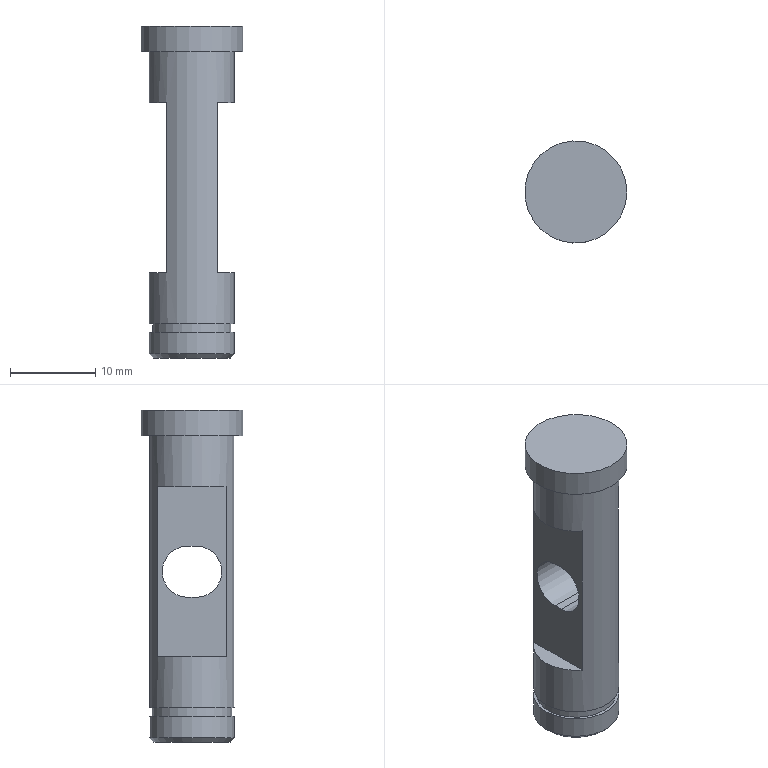Part | NX | features BREP 1, DATUM_CSYS 1 | 1 solid | 20 faces | box 12 x 12 x 39 mm | volume 2499 mm3 | plane 13 | cylinder 6 | cone 1 | commonest cylinder face diameters 6 x2 10 x2 9.3 x1 12 x1
STEP:
#1=CARTESIAN_POINT('',(6.,0.,3.));
#2=VERTEX_POINT('',#1);
#3=CARTESIAN_POINT('',(0.,0.,3.));
#4=DIRECTION('',(0.,0.,1.));
#5=DIRECTION('',(1.,0.,0.));
#6=AXIS2_PLACEMENT_3D('',#3,#4,#5);
#7=CIRCLE('',#6,6.);
#8=EDGE_CURVE('',#2,#2,#7,.T.);
#9=ORIENTED_EDGE('',*,*,#8,.T.);
#10=EDGE_LOOP('',(#9));
#11=FACE_BOUND('',#10,.T.);
#12=CARTESIAN_POINT('',(0.,0.,3.));
#13=DIRECTION('',(0.,0.,1.));
#14=DIRECTION('',(-1.,0.,0.));
#15=AXIS2_PLACEMENT_3D('',#12,#13,#14);
#16=PLANE('',#15);
#17=ADVANCED_FACE('',(#11),#16,.T.);
#18=CARTESIAN_POINT('',(6.,0.,0.));
#19=VERTEX_POINT('',#18);
#20=CARTESIAN_POINT('',(0.,0.,0.));
#21=DIRECTION('',(0.,0.,1.));
#22=DIRECTION('',(1.,0.,0.));
#23=AXIS2_PLACEMENT_3D('',#20,#21,#22);
#24=CIRCLE('',#23,6.);
#25=EDGE_CURVE('',#19,#19,#24,.T.);
#26=ORIENTED_EDGE('',*,*,#25,.T.);
#27=CARTESIAN_POINT('',(6.,0.,0.));
#28=DIRECTION('',(0.,0.,1.));
#29=VECTOR('',#28,1000.);
#30=LINE('',#27,#29);
#31=EDGE_CURVE('',#19,#2,#30,.T.);
#32=ORIENTED_EDGE('',*,*,#31,.T.);
#33=ORIENTED_EDGE('',*,*,#8,.F.);
#34=ORIENTED_EDGE('',*,*,#31,.F.);
#35=EDGE_LOOP('',(#26,#32,#33,#34));
#36=FACE_BOUND('',#35,.T.);
#37=CARTESIAN_POINT('',(0.,0.,0.));
#38=DIRECTION('',(0.,0.,1.));
#39=DIRECTION('',(-1.,0.,0.));
#40=AXIS2_PLACEMENT_3D('',#37,#38,#39);
#41=CYLINDRICAL_SURFACE('',#40,6.);
#42=ADVANCED_FACE('',(#36),#41,.T.);
#43=ORIENTED_EDGE('',*,*,#25,.F.);
#44=EDGE_LOOP('',(#43));
#45=FACE_BOUND('',#44,.T.);
#46=CARTESIAN_POINT('',(5.,0.,0.));
#47=VERTEX_POINT('',#46);
#48=CARTESIAN_POINT('',(0.,0.,0.));
#49=DIRECTION('',(0.,0.,-1.));
#50=DIRECTION('',(1.,0.,0.));
#51=AXIS2_PLACEMENT_3D('',#48,#49,#50);
#52=CIRCLE('',#51,5.);
#53=EDGE_CURVE('',#47,#47,#52,.T.);
#54=ORIENTED_EDGE('',*,*,#53,.F.);
#55=EDGE_LOOP('',(#54));
#56=FACE_BOUND('',#55,.T.);
#57=CARTESIAN_POINT('',(0.,0.,0.));
#58=DIRECTION('',(0.,0.,1.));
#59=DIRECTION('',(-1.,0.,0.));
#60=AXIS2_PLACEMENT_3D('',#57,#58,#59);
#61=PLANE('',#60);
#62=ADVANCED_FACE('',(#45,#56),#61,.F.);
#63=CARTESIAN_POINT('',(3.,4.,-6.));
#64=VERTEX_POINT('',#63);
#65=CARTESIAN_POINT('',(5.,0.,-6.));
#66=VERTEX_POINT('',#65);
#67=CARTESIAN_POINT('',(0.,0.,-6.));
#68=DIRECTION('',(0.,0.,-1.));
#69=DIRECTION('',(0.6,0.8,0.));
#70=AXIS2_PLACEMENT_3D('',#67,#68,#69);
#71=CIRCLE('',#70,5.);
#72=EDGE_CURVE('',#64,#66,#71,.T.);
#73=ORIENTED_EDGE('',*,*,#72,.T.);
#74=CARTESIAN_POINT('',(3.,-4.,-6.));
#75=VERTEX_POINT('',#74);
#76=CARTESIAN_POINT('',(0.,0.,-6.));
#77=DIRECTION('',(0.,0.,-1.));
#78=DIRECTION('',(1.,0.,0.));
#79=AXIS2_PLACEMENT_3D('',#76,#77,#78);
#80=CIRCLE('',#79,5.);
#81=EDGE_CURVE('',#66,#75,#80,.T.);
#82=ORIENTED_EDGE('',*,*,#81,.T.);
#83=CARTESIAN_POINT('',(3.,4.,-6.));
#84=DIRECTION('',(0.,-1.,0.));
#85=VECTOR('',#84,1000.);
#86=LINE('',#83,#85);
#87=EDGE_CURVE('',#64,#75,#86,.T.);
#88=ORIENTED_EDGE('',*,*,#87,.F.);
#89=EDGE_LOOP('',(#73,#82,#88));
#90=FACE_BOUND('',#89,.T.);
#91=CARTESIAN_POINT('',(6.893,0.,-6.));
#92=DIRECTION('',(0.,0.,1.));
#93=DIRECTION('',(1.,0.,0.));
#94=AXIS2_PLACEMENT_3D('',#91,#92,#93);
#95=PLANE('',#94);
#96=ADVANCED_FACE('',(#90),#95,.F.);
#97=CARTESIAN_POINT('',(3.,-4.,-26.));
#98=VERTEX_POINT('',#97);
#99=CARTESIAN_POINT('',(3.,-4.,-6.));
#100=DIRECTION('',(0.,0.,-1.));
#101=VECTOR('',#100,1000.);
#102=LINE('',#99,#101);
#103=EDGE_CURVE('',#75,#98,#102,.T.);
#104=ORIENTED_EDGE('',*,*,#103,.T.);
#105=CARTESIAN_POINT('',(3.,4.,-26.));
#106=VERTEX_POINT('',#105);
#107=CARTESIAN_POINT('',(3.,-4.,-26.));
#108=DIRECTION('',(0.,1.,0.));
#109=VECTOR('',#108,1000.);
#110=LINE('',#107,#109);
#111=EDGE_CURVE('',#98,#106,#110,.T.);
#112=ORIENTED_EDGE('',*,*,#111,.T.);
#113=CARTESIAN_POINT('',(3.,4.,-26.));
#114=DIRECTION('',(0.,0.,1.));
#115=VECTOR('',#114,1000.);
#116=LINE('',#113,#115);
#117=EDGE_CURVE('',#106,#64,#116,.T.);
#118=ORIENTED_EDGE('',*,*,#117,.T.);
#119=ORIENTED_EDGE('',*,*,#87,.T.);
#120=EDGE_LOOP('',(#104,#112,#118,#119));
#121=FACE_BOUND('',#120,.T.);
#122=CARTESIAN_POINT('',(3.,0.5,-19.));
#123=VERTEX_POINT('',#122);
#124=CARTESIAN_POINT('',(3.,0.5,-13.));
#125=VERTEX_POINT('',#124);
#126=CARTESIAN_POINT('',(3.,0.5,-16.));
#127=DIRECTION('',(1.,0.,0.));
#128=DIRECTION('',(0.,0.,-1.));
#129=AXIS2_PLACEMENT_3D('',#126,#127,#128);
#130=CIRCLE('',#129,3.);
#131=EDGE_CURVE('',#123,#125,#130,.T.);
#132=ORIENTED_EDGE('',*,*,#131,.F.);
#133=CARTESIAN_POINT('',(3.,-0.5,-19.));
#134=VERTEX_POINT('',#133);
#135=CARTESIAN_POINT('',(3.,-0.5,-19.));
#136=DIRECTION('',(0.,1.,0.));
#137=VECTOR('',#136,1000.);
#138=LINE('',#135,#137);
#139=EDGE_CURVE('',#134,#123,#138,.T.);
#140=ORIENTED_EDGE('',*,*,#139,.F.);
#141=CARTESIAN_POINT('',(3.,-0.5,-13.));
#142=VERTEX_POINT('',#141);
#143=CARTESIAN_POINT('',(3.,-0.5,-16.));
#144=DIRECTION('',(1.,0.,0.));
#145=DIRECTION('',(0.,0.,1.));
#146=AXIS2_PLACEMENT_3D('',#143,#144,#145);
#147=CIRCLE('',#146,3.);
#148=EDGE_CURVE('',#142,#134,#147,.T.);
#149=ORIENTED_EDGE('',*,*,#148,.F.);
#150=CARTESIAN_POINT('',(3.,0.5,-13.));
#151=DIRECTION('',(0.,-1.,0.));
#152=VECTOR('',#151,1000.);
#153=LINE('',#150,#152);
#154=EDGE_CURVE('',#125,#142,#153,.T.);
#155=ORIENTED_EDGE('',*,*,#154,.F.);
#156=EDGE_LOOP('',(#132,#140,#149,#155));
#157=FACE_BOUND('',#156,.T.);
#158=CARTESIAN_POINT('',(3.,0.,-21.759));
#159=DIRECTION('',(-1.,0.,0.));
#160=DIRECTION('',(0.,0.,1.));
#161=AXIS2_PLACEMENT_3D('',#158,#159,#160);
#162=PLANE('',#161);
#163=ADVANCED_FACE('',(#121,#157),#162,.F.);
#164=CARTESIAN_POINT('',(-3.,4.,-6.));
#165=VERTEX_POINT('',#164);
#166=CARTESIAN_POINT('',(-3.,4.,-26.));
#167=VERTEX_POINT('',#166);
#168=CARTESIAN_POINT('',(-3.,4.,-6.));
#169=DIRECTION('',(0.,0.,-1.));
#170=VECTOR('',#169,1000.);
#171=LINE('',#168,#170);
#172=EDGE_CURVE('',#165,#167,#171,.T.);
#173=ORIENTED_EDGE('',*,*,#172,.T.);
#174=CARTESIAN_POINT('',(-3.,-4.,-26.));
#175=VERTEX_POINT('',#174);
#176=CARTESIAN_POINT('',(-3.,4.,-26.));
#177=DIRECTION('',(0.,-1.,0.));
#178=VECTOR('',#177,1000.);
#179=LINE('',#176,#178);
#180=EDGE_CURVE('',#167,#175,#179,.T.);
#181=ORIENTED_EDGE('',*,*,#180,.T.);
#182=CARTESIAN_POINT('',(-3.,-4.,-6.));
#183=VERTEX_POINT('',#182);
#184=CARTESIAN_POINT('',(-3.,-4.,-26.));
#185=DIRECTION('',(0.,0.,1.));
#186=VECTOR('',#185,1000.);
#187=LINE('',#184,#186);
#188=EDGE_CURVE('',#175,#183,#187,.T.);
#189=ORIENTED_EDGE('',*,*,#188,.T.);
#190=CARTESIAN_POINT('',(-3.,4.,-6.));
#191=DIRECTION('',(0.,-1.,0.));
#192=VECTOR('',#191,1000.);
#193=LINE('',#190,#192);
#194=EDGE_CURVE('',#165,#183,#193,.T.);
#195=ORIENTED_EDGE('',*,*,#194,.F.);
#196=EDGE_LOOP('',(#173,#181,#189,#195));
#197=FACE_BOUND('',#196,.T.);
#198=CARTESIAN_POINT('',(-3.,0.5,-13.));
#199=VERTEX_POINT('',#198);
#200=CARTESIAN_POINT('',(-3.,0.5,-19.));
#201=VERTEX_POINT('',#200);
#202=CARTESIAN_POINT('',(-3.,0.5,-16.));
#203=DIRECTION('',(-1.,0.,0.));
#204=DIRECTION('',(0.,0.,1.));
#205=AXIS2_PLACEMENT_3D('',#202,#203,#204);
#206=CIRCLE('',#205,3.);
#207=EDGE_CURVE('',#199,#201,#206,.T.);
#208=ORIENTED_EDGE('',*,*,#207,.F.);
#209=CARTESIAN_POINT('',(-3.,-0.5,-13.));
#210=VERTEX_POINT('',#209);
#211=CARTESIAN_POINT('',(-3.,-0.5,-13.));
#212=DIRECTION('',(0.,1.,0.));
#213=VECTOR('',#212,1000.);
#214=LINE('',#211,#213);
#215=EDGE_CURVE('',#210,#199,#214,.T.);
#216=ORIENTED_EDGE('',*,*,#215,.F.);
#217=CARTESIAN_POINT('',(-3.,-0.5,-19.));
#218=VERTEX_POINT('',#217);
#219=CARTESIAN_POINT('',(-3.,-0.5,-16.));
#220=DIRECTION('',(-1.,0.,0.));
#221=DIRECTION('',(0.,0.,-1.));
#222=AXIS2_PLACEMENT_3D('',#219,#220,#221);
#223=CIRCLE('',#222,3.);
#224=EDGE_CURVE('',#218,#210,#223,.T.);
#225=ORIENTED_EDGE('',*,*,#224,.F.);
#226=CARTESIAN_POINT('',(-3.,0.5,-19.));
#227=DIRECTION('',(0.,-1.,0.));
#228=VECTOR('',#227,1000.);
#229=LINE('',#226,#228);
#230=EDGE_CURVE('',#201,#218,#229,.T.);
#231=ORIENTED_EDGE('',*,*,#230,.F.);
#232=EDGE_LOOP('',(#208,#216,#225,#231));
#233=FACE_BOUND('',#232,.T.);
#234=CARTESIAN_POINT('',(-3.,0.,-21.759));
#235=DIRECTION('',(1.,0.,0.));
#236=DIRECTION('',(0.,0.,-1.));
#237=AXIS2_PLACEMENT_3D('',#234,#235,#236);
#238=PLANE('',#237);
#239=ADVANCED_FACE('',(#197,#233),#238,.F.);
#240=CARTESIAN_POINT('',(0.,0.,-6.));
#241=DIRECTION('',(0.,0.,-1.));
#242=DIRECTION('',(-0.6,-0.8,0.));
#243=AXIS2_PLACEMENT_3D('',#240,#241,#242);
#244=CIRCLE('',#243,5.);
#245=EDGE_CURVE('',#183,#165,#244,.T.);
#246=ORIENTED_EDGE('',*,*,#245,.T.);
#247=ORIENTED_EDGE('',*,*,#194,.T.);
#248=EDGE_LOOP('',(#246,#247));
#249=FACE_BOUND('',#248,.T.);
#250=CARTESIAN_POINT('',(-6.923,0.,-6.));
#251=DIRECTION('',(0.,0.,1.));
#252=DIRECTION('',(1.,0.,0.));
#253=AXIS2_PLACEMENT_3D('',#250,#251,#252);
#254=PLANE('',#253);
#255=ADVANCED_FACE('',(#249),#254,.F.);
#256=ORIENTED_EDGE('',*,*,#154,.T.);
#257=CARTESIAN_POINT('',(-3.,-0.5,-13.));
#258=DIRECTION('',(1.,0.,0.));
#259=VECTOR('',#258,1000.);
#260=LINE('',#257,#259);
#261=EDGE_CURVE('',#210,#142,#260,.T.);
#262=ORIENTED_EDGE('',*,*,#261,.F.);
#263=ORIENTED_EDGE('',*,*,#215,.T.);
#264=CARTESIAN_POINT('',(-3.,0.5,-13.));
#265=DIRECTION('',(1.,0.,0.));
#266=VECTOR('',#265,1000.);
#267=LINE('',#264,#266);
#268=EDGE_CURVE('',#199,#125,#267,.T.);
#269=ORIENTED_EDGE('',*,*,#268,.T.);
#270=EDGE_LOOP('',(#256,#262,#263,#269));
#271=FACE_BOUND('',#270,.T.);
#272=CARTESIAN_POINT('',(3.,0.,-13.));
#273=DIRECTION('',(0.,0.,1.));
#274=DIRECTION('',(0.,1.,0.));
#275=AXIS2_PLACEMENT_3D('',#272,#273,#274);
#276=PLANE('',#275);
#277=ADVANCED_FACE('',(#271),#276,.F.);
#278=ORIENTED_EDGE('',*,*,#148,.T.);
#279=CARTESIAN_POINT('',(-3.,-0.5,-19.));
#280=DIRECTION('',(1.,0.,0.));
#281=VECTOR('',#280,1000.);
#282=LINE('',#279,#281);
#283=EDGE_CURVE('',#218,#134,#282,.T.);
#284=ORIENTED_EDGE('',*,*,#283,.F.);
#285=ORIENTED_EDGE('',*,*,#224,.T.);
#286=ORIENTED_EDGE('',*,*,#261,.T.);
#287=EDGE_LOOP('',(#278,#284,#285,#286));
#288=FACE_BOUND('',#287,.T.);
#289=CARTESIAN_POINT('',(-47.,-0.5,-16.));
#290=DIRECTION('',(1.,0.,0.));
#291=DIRECTION('',(0.,0.,-1.));
#292=AXIS2_PLACEMENT_3D('',#289,#290,#291);
#293=CYLINDRICAL_SURFACE('',#292,3.);
#294=ADVANCED_FACE('',(#288),#293,.F.);
#295=ORIENTED_EDGE('',*,*,#139,.T.);
#296=CARTESIAN_POINT('',(-3.,0.5,-19.));
#297=DIRECTION('',(1.,0.,0.));
#298=VECTOR('',#297,1000.);
#299=LINE('',#296,#298);
#300=EDGE_CURVE('',#201,#123,#299,.T.);
#301=ORIENTED_EDGE('',*,*,#300,.F.);
#302=ORIENTED_EDGE('',*,*,#230,.T.);
#303=ORIENTED_EDGE('',*,*,#283,.T.);
#304=EDGE_LOOP('',(#295,#301,#302,#303));
#305=FACE_BOUND('',#304,.T.);
#306=CARTESIAN_POINT('',(3.,0.,-19.));
#307=DIRECTION('',(0.,0.,-1.));
#308=DIRECTION('',(0.,-1.,0.));
#309=AXIS2_PLACEMENT_3D('',#306,#307,#308);
#310=PLANE('',#309);
#311=ADVANCED_FACE('',(#305),#310,.F.);
#312=ORIENTED_EDGE('',*,*,#131,.T.);
#313=ORIENTED_EDGE('',*,*,#268,.F.);
#314=ORIENTED_EDGE('',*,*,#207,.T.);
#315=ORIENTED_EDGE('',*,*,#300,.T.);
#316=EDGE_LOOP('',(#312,#313,#314,#315));
#317=FACE_BOUND('',#316,.T.);
#318=CARTESIAN_POINT('',(-47.,0.5,-16.));
#319=DIRECTION('',(1.,0.,0.));
#320=DIRECTION('',(0.,0.,1.));
#321=AXIS2_PLACEMENT_3D('',#318,#319,#320);
#322=CYLINDRICAL_SURFACE('',#321,3.);
#323=ADVANCED_FACE('',(#317),#322,.F.);
#324=ORIENTED_EDGE('',*,*,#111,.F.);
#325=CARTESIAN_POINT('',(5.,0.,-26.));
#326=VERTEX_POINT('',#325);
#327=CARTESIAN_POINT('',(0.,0.,-26.));
#328=DIRECTION('',(0.,0.,-1.));
#329=DIRECTION('',(1.,0.,0.));
#330=AXIS2_PLACEMENT_3D('',#327,#328,#329);
#331=CIRCLE('',#330,5.);
#332=EDGE_CURVE('',#326,#98,#331,.T.);
#333=ORIENTED_EDGE('',*,*,#332,.F.);
#334=CARTESIAN_POINT('',(0.,0.,-26.));
#335=DIRECTION('',(0.,0.,-1.));
#336=DIRECTION('',(0.6,0.8,0.));
#337=AXIS2_PLACEMENT_3D('',#334,#335,#336);
#338=CIRCLE('',#337,5.);
#339=EDGE_CURVE('',#106,#326,#338,.T.);
#340=ORIENTED_EDGE('',*,*,#339,.F.);
#341=EDGE_LOOP('',(#324,#333,#340));
#342=FACE_BOUND('',#341,.T.);
#343=CARTESIAN_POINT('',(-0.000000011,-0.000000008,-26.));
#344=DIRECTION('',(0.,0.,-1.));
#345=DIRECTION('',(-0.6,0.8,0.));
#346=AXIS2_PLACEMENT_3D('',#343,#344,#345);
#347=PLANE('',#346);
#348=ADVANCED_FACE('',(#342),#347,.F.);
#349=CARTESIAN_POINT('',(4.5,0.,-36.));
#350=VERTEX_POINT('',#349);
#351=CARTESIAN_POINT('',(0.,0.,-36.));
#352=DIRECTION('',(0.,0.,1.));
#353=DIRECTION('',(1.,0.,0.));
#354=AXIS2_PLACEMENT_3D('',#351,#352,#353);
#355=CIRCLE('',#354,4.5);
#356=EDGE_CURVE('',#350,#350,#355,.T.);
#357=ORIENTED_EDGE('',*,*,#356,.F.);
#358=EDGE_LOOP('',(#357));
#359=FACE_BOUND('',#358,.T.);
#360=CARTESIAN_POINT('',(0.,0.,-36.));
#361=DIRECTION('',(0.,0.,-1.));
#362=DIRECTION('',(-0.6,0.8,0.));
#363=AXIS2_PLACEMENT_3D('',#360,#361,#362);
#364=PLANE('',#363);
#365=ADVANCED_FACE('',(#359),#364,.T.);
#366=ORIENTED_EDGE('',*,*,#180,.F.);
#367=CARTESIAN_POINT('',(0.,0.,-26.));
#368=DIRECTION('',(0.,0.,-1.));
#369=DIRECTION('',(-0.6,-0.8,0.));
#370=AXIS2_PLACEMENT_3D('',#367,#368,#369);
#371=CIRCLE('',#370,5.);
#372=EDGE_CURVE('',#175,#167,#371,.T.);
#373=ORIENTED_EDGE('',*,*,#372,.F.);
#374=EDGE_LOOP('',(#366,#373));
#375=FACE_BOUND('',#374,.T.);
#376=CARTESIAN_POINT('',(-0.000000011,-0.000000008,-26.));
#377=DIRECTION('',(0.,0.,-1.));
#378=DIRECTION('',(-0.6,0.8,0.));
#379=AXIS2_PLACEMENT_3D('',#376,#377,#378);
#380=PLANE('',#379);
#381=ADVANCED_FACE('',(#375),#380,.F.);
#382=CARTESIAN_POINT('',(5.,0.,-35.5));
#383=VERTEX_POINT('',#382);
#384=CARTESIAN_POINT('',(4.5,0.,-36.));
#385=DIRECTION('',(0.7071,0.,0.7071));
#386=VECTOR('',#385,1000.);
#387=LINE('',#384,#386);
#388=EDGE_CURVE('',#350,#383,#387,.T.);
#389=ORIENTED_EDGE('',*,*,#388,.T.);
#390=CARTESIAN_POINT('',(0.,0.,-35.5));
#391=DIRECTION('',(0.,0.,1.));
#392=DIRECTION('',(1.,0.,0.));
#393=AXIS2_PLACEMENT_3D('',#390,#391,#392);
#394=CIRCLE('',#393,5.);
#395=EDGE_CURVE('',#383,#383,#394,.T.);
#396=ORIENTED_EDGE('',*,*,#395,.F.);
#397=ORIENTED_EDGE('',*,*,#388,.F.);
#398=ORIENTED_EDGE('',*,*,#356,.T.);
#399=EDGE_LOOP('',(#389,#396,#397,#398));
#400=FACE_BOUND('',#399,.T.);
#401=CARTESIAN_POINT('',(0.,0.,-36.));
#402=DIRECTION('',(0.,0.,1.));
#403=DIRECTION('',(-1.,0.,0.));
#404=AXIS2_PLACEMENT_3D('',#401,#402,#403);
#405=CONICAL_SURFACE('',#404,4.5,0.7854);
#406=ADVANCED_FACE('',(#400),#405,.T.);
#407=ORIENTED_EDGE('',*,*,#53,.T.);
#408=CARTESIAN_POINT('',(5.,0.,0.));
#409=DIRECTION('',(0.,0.,-1.));
#410=VECTOR('',#409,1000.);
#411=LINE('',#408,#410);
#412=EDGE_CURVE('',#47,#66,#411,.T.);
#413=ORIENTED_EDGE('',*,*,#412,.T.);
#414=ORIENTED_EDGE('',*,*,#72,.F.);
#415=ORIENTED_EDGE('',*,*,#117,.F.);
#416=ORIENTED_EDGE('',*,*,#339,.T.);
#417=CARTESIAN_POINT('',(5.,0.,-32.));
#418=VERTEX_POINT('',#417);
#419=CARTESIAN_POINT('',(5.,0.,-26.));
#420=DIRECTION('',(0.,0.,-1.));
#421=VECTOR('',#420,1000.);
#422=LINE('',#419,#421);
#423=EDGE_CURVE('',#326,#418,#422,.T.);
#424=ORIENTED_EDGE('',*,*,#423,.T.);
#425=CARTESIAN_POINT('',(0.,0.,-32.));
#426=DIRECTION('',(0.,0.,-1.));
#427=DIRECTION('',(1.,0.,0.));
#428=AXIS2_PLACEMENT_3D('',#425,#426,#427);
#429=CIRCLE('',#428,5.);
#430=EDGE_CURVE('',#418,#418,#429,.T.);
#431=ORIENTED_EDGE('',*,*,#430,.F.);
#432=ORIENTED_EDGE('',*,*,#423,.F.);
#433=ORIENTED_EDGE('',*,*,#332,.T.);
#434=ORIENTED_EDGE('',*,*,#103,.F.);
#435=ORIENTED_EDGE('',*,*,#81,.F.);
#436=ORIENTED_EDGE('',*,*,#412,.F.);
#437=EDGE_LOOP('',(#407,#413,#414,#415,#416,#424,#431,#432,#433,#434,#435,#436));
#438=FACE_BOUND('',#437,.T.);
#439=ORIENTED_EDGE('',*,*,#172,.F.);
#440=ORIENTED_EDGE('',*,*,#245,.F.);
#441=ORIENTED_EDGE('',*,*,#188,.F.);
#442=ORIENTED_EDGE('',*,*,#372,.T.);
#443=EDGE_LOOP('',(#439,#440,#441,#442));
#444=FACE_BOUND('',#443,.T.);
#445=CARTESIAN_POINT('',(0.,0.,0.));
#446=DIRECTION('',(0.,0.,-1.));
#447=DIRECTION('',(-1.,0.,0.));
#448=AXIS2_PLACEMENT_3D('',#445,#446,#447);
#449=CYLINDRICAL_SURFACE('',#448,5.);
#450=ADVANCED_FACE('',(#438,#444),#449,.T.);
#451=ORIENTED_EDGE('',*,*,#395,.T.);
#452=CARTESIAN_POINT('',(5.,0.,-33.));
#453=VERTEX_POINT('',#452);
#454=CARTESIAN_POINT('',(5.,0.,-33.));
#455=DIRECTION('',(0.,0.,-1.));
#456=VECTOR('',#455,1000.);
#457=LINE('',#454,#456);
#458=EDGE_CURVE('',#453,#383,#457,.T.);
#459=ORIENTED_EDGE('',*,*,#458,.F.);
#460=CARTESIAN_POINT('',(0.,0.,-33.));
#461=DIRECTION('',(0.,0.,-1.));
#462=DIRECTION('',(1.,0.,0.));
#463=AXIS2_PLACEMENT_3D('',#460,#461,#462);
#464=CIRCLE('',#463,5.);
#465=EDGE_CURVE('',#453,#453,#464,.T.);
#466=ORIENTED_EDGE('',*,*,#465,.T.);
#467=ORIENTED_EDGE('',*,*,#458,.T.);
#468=EDGE_LOOP('',(#451,#459,#466,#467));
#469=FACE_BOUND('',#468,.T.);
#470=CARTESIAN_POINT('',(0.,0.,0.));
#471=DIRECTION('',(0.,0.,-1.));
#472=DIRECTION('',(-1.,0.,0.));
#473=AXIS2_PLACEMENT_3D('',#470,#471,#472);
#474=CYLINDRICAL_SURFACE('',#473,5.);
#475=ADVANCED_FACE('',(#469),#474,.T.);
#476=ORIENTED_EDGE('',*,*,#430,.T.);
#477=EDGE_LOOP('',(#476));
#478=FACE_BOUND('',#477,.T.);
#479=CARTESIAN_POINT('',(0.,-4.65,-32.));
#480=VERTEX_POINT('',#479);
#481=CARTESIAN_POINT('',(0.,0.,-32.));
#482=DIRECTION('',(0.,0.,1.));
#483=DIRECTION('',(0.,-1.,0.));
#484=AXIS2_PLACEMENT_3D('',#481,#482,#483);
#485=CIRCLE('',#484,4.65);
#486=EDGE_CURVE('',#480,#480,#485,.T.);
#487=ORIENTED_EDGE('',*,*,#486,.T.);
#488=EDGE_LOOP('',(#487));
#489=FACE_BOUND('',#488,.T.);
#490=CARTESIAN_POINT('',(0.,0.,-32.));
#491=DIRECTION('',(0.,0.,-1.));
#492=DIRECTION('',(0.,1.,0.));
#493=AXIS2_PLACEMENT_3D('',#490,#491,#492);
#494=PLANE('',#493);
#495=ADVANCED_FACE('',(#478,#489),#494,.T.);
#496=CARTESIAN_POINT('',(0.,-4.65,-33.));
#497=VERTEX_POINT('',#496);
#498=CARTESIAN_POINT('',(0.,-4.65,-32.));
#499=DIRECTION('',(0.,0.,-1.));
#500=VECTOR('',#499,1000.);
#501=LINE('',#498,#500);
#502=EDGE_CURVE('',#480,#497,#501,.T.);
#503=ORIENTED_EDGE('',*,*,#502,.T.);
#504=CARTESIAN_POINT('',(0.,0.,-33.));
#505=DIRECTION('',(0.,0.,1.));
#506=DIRECTION('',(0.,-1.,0.));
#507=AXIS2_PLACEMENT_3D('',#504,#505,#506);
#508=CIRCLE('',#507,4.65);
#509=EDGE_CURVE('',#497,#497,#508,.T.);
#510=ORIENTED_EDGE('',*,*,#509,.T.);
#511=ORIENTED_EDGE('',*,*,#502,.F.);
#512=ORIENTED_EDGE('',*,*,#486,.F.);
#513=EDGE_LOOP('',(#503,#510,#511,#512));
#514=FACE_BOUND('',#513,.T.);
#515=CARTESIAN_POINT('',(0.,0.,-32.));
#516=DIRECTION('',(0.,0.,-1.));
#517=DIRECTION('',(0.,1.,0.));
#518=AXIS2_PLACEMENT_3D('',#515,#516,#517);
#519=CYLINDRICAL_SURFACE('',#518,4.65);
#520=ADVANCED_FACE('',(#514),#519,.T.);
#521=ORIENTED_EDGE('',*,*,#465,.F.);
#522=EDGE_LOOP('',(#521));
#523=FACE_BOUND('',#522,.T.);
#524=ORIENTED_EDGE('',*,*,#509,.F.);
#525=EDGE_LOOP('',(#524));
#526=FACE_BOUND('',#525,.T.);
#527=CARTESIAN_POINT('',(0.,0.,-33.));
#528=DIRECTION('',(0.,0.,1.));
#529=DIRECTION('',(0.,1.,0.));
#530=AXIS2_PLACEMENT_3D('',#527,#528,#529);
#531=PLANE('',#530);
#532=ADVANCED_FACE('',(#523,#526),#531,.T.);
#533=CLOSED_SHELL('',(#17,#42,#62,#96,#163,#239,#255,#277,#294,#311,#323,#348,#365,#381,#406,#450,#475,#495,#520,#532));
#534=MANIFOLD_SOLID_BREP('',#533);
#535=(LENGTH_UNIT()NAMED_UNIT(*)SI_UNIT(.MILLI.,.METRE.));
#536=UNCERTAINTY_MEASURE_WITH_UNIT(LENGTH_MEASURE(0.00001),#535,'','');
#537=(NAMED_UNIT(*)PLANE_ANGLE_UNIT()SI_UNIT($,.RADIAN.));
#538=(NAMED_UNIT(*)SI_UNIT($,.STERADIAN.)SOLID_ANGLE_UNIT());
#539=(GEOMETRIC_REPRESENTATION_CONTEXT(3)GLOBAL_UNCERTAINTY_ASSIGNED_CONTEXT((#536))GLOBAL_UNIT_ASSIGNED_CONTEXT((#535,#537,#538))REPRESENTATION_CONTEXT('',''));
#540=ADVANCED_BREP_SHAPE_REPRESENTATION('',(#534),#539);